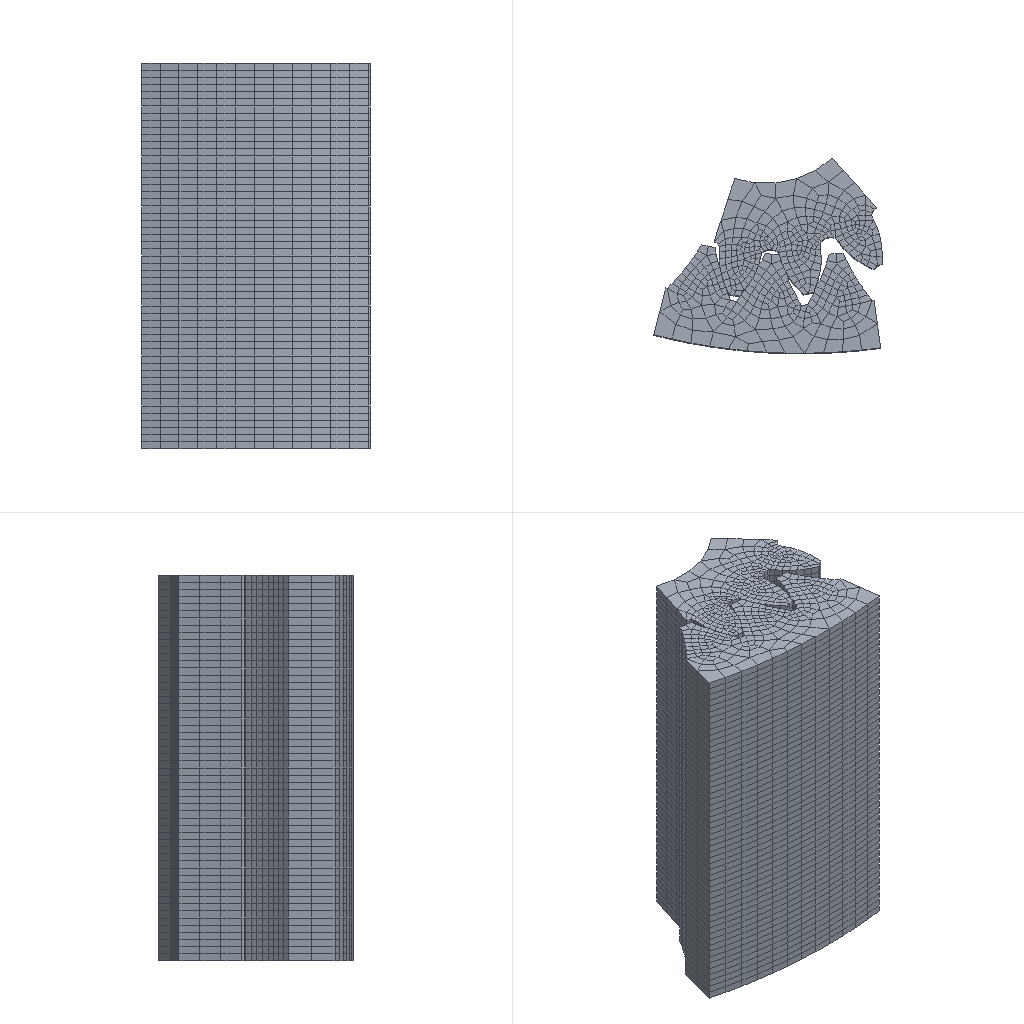Simulation study | abaqus
Set-up summary:
category,name,step,type,value,unit,region
solver,abaqus
solver,version,,,Abaqus/Standard 2020
units,not stated in the deck,,not stated
analysis,deck,,static,static
load_step,Step-1,Step-1,static
load_step,requested,,,1
mesh,nodes,,,31130
mesh,elements,,,26406
element_type,C3D8R,,solid,26406
load,load commands in deck,,count,1
bc,support commands in deck,,count,6
material,MATERIAL-1,,in results
check,setup vs results,,match,"per instance, exact: element labels, types and connectivity; labels of the nodes the elements use; coordinates of those nodes at SINGLE_PRECISION in 1 of 2 instance(s)"
Abaqus input file, long lists of numbers shortened:
*Heading
** Job name: Job-1 Model name: Model-1
** Generated by: Abaqus/CAE 2020
*Preprint, echo=NO, model=NO, history=NO, contact=NO
**
** PARTS
**
*Part, name=work-1
*Node
      1,  -37.365,   11.966,         13.5
      2,  -34.285,   8.516,         13.5
** (17378 more lines like these left out)
*Element, type=C3D8R
    1,    52,    85,    55,     2,   368,   401,   371,   318
    2,    55,    85,   265,   199,   371,   401,   581,   515
** (14956 more lines like these left out)
*Nset, nset=Set-1, generate
     1,  17380,      1
*Elset, elset=Set-1, generate
     1,  14958,      1
** Section: Section-1
*Solid Section, elset=Set-1, material=Material-1
,
*End Part
**
*Part, name=work-2
*Node
      1,  -45.957,  -1.201,        -13.5
      2,  -41.979,  -1.625,        -13.5
** (13748 more lines like these left out)
*Element, type=C3D8R
    1,   202,   195,   204,   210,   452,   445,   454,   460
    2,    76,   245,   183,   230,   326,   495,   433,   480
** (11446 more lines like these left out)
*Nset, nset=Set-1, generate
     1,  13750,      1
*Elset, elset=Set-1, generate
     1,  11448,      1
** Section: Section-1
*Solid Section, elset=Set-1, material=Material-1
,
*End Part
**
**
** ASSEMBLY
**
*Assembly, name=Assembly
**
*Instance, name=work-1-1, part=work-1
*End Instance
**
*Instance, name=work-2-1, part=work-2
*End Instance
**
*Node
      1,  -42.027,   17.188, 6.75015599e-14
*Nset, nset=Set-1, instance=work-2-1
     1,     2,     3,     4,     5,    29,    30,    31,    32,    33,    34,    35,    36,   251,   252,   253
   254,   255,   279,   280,   281,   282,   283,   284,   285,   286,   501,   502,   503,   504,   505,   529
** (43 more lines like these left out)
*Elset, elset=Set-1, instance=work-2-1
    26,   161,   167,   175,   177,   188,   191,   192,   196,   200,   205,   207,   238,   373,   379,   387
   389,   400,   403,   404,   408,   412,   417,   419,   450,   585,   591,   599,   601,   612,   615,   616
** (39 more lines like these left out)
*Nset, nset=Set-3
 1,
*Nset, nset=Set-4
 1,
*Nset, nset=Set-5, instance=work-1-1
     1,     2,     3,     4,     5,     6,     7,     8,     9,    10,    11,    12,    13,    14,    15,    16
    17,    18,    19,    20,    21,    22,    23,    24,    25,    26,    27,    28,    29,    30,    31,    32
** (38 more lines like these left out)
*Elset, elset=Set-5, instance=work-1-1
     1,     2,     3,     4,     5,     6,     7,     8,     9,    10,    11,    12,    13,    14,    15,    16
    17,    18,    19,    20,    21,    22,    23,    24,    25,    26,    27,    28,    29,    30,    31,    32
** (33 more lines like these left out)
*Nset, nset=Set-6
 1,
*Nset, nset=m_Set-2
 1,
*Elset, elset=_m_Surf-2_S6, internal, instance=work-1-1
     1,     5,     7,    11,    20,    21,    25,    39,    89,   105,   112,   161,   260,   278,   282,   284
   288,   297,   298,   302,   316,   366,   382,   389,   438,   537,   555,   559,   561,   565,   574,   575
** (42 more lines like these left out)
*Elset, elset=_m_Surf-2_S5, internal, instance=work-1-1
    11,    14,    17,    21,    26,    31,    33,    39,    56,    57,    59,    61,    62,    84,    89,    94
    95,   107,   110,   116,   120,   160,   161,   288,   291,   294,   298,   303,   308,   310,   316,   333
** (76 more lines like these left out)
*Elset, elset=_m_Surf-2_S3, internal, instance=work-1-1
    10,    16,    19,    27,    50,    58,    71,   162,   287,   293,   296,   304,   327,   335,   348,   439
   564,   570,   573,   581,   604,   612,   625,   716,   841,   847,   850,   858,   881,   889,   902,   993
** (25 more lines like these left out)
*Elset, elset=_m_Surf-2_S4, internal, instance=work-1-1
    12,    29,    34,    41,    44,    49,    51,    52,    53,    64,    65,    68,    70,    72,    80,    82
    96,    97,   108,   109,   289,   306,   311,   318,   321,   326,   328,   329,   330,   341,   342,   345
** (66 more lines like these left out)
*Surface, type=ELEMENT, name=m_Surf-2
_m_Surf-2_S6, S6
_m_Surf-2_S5, S5
_m_Surf-2_S4, S4
_m_Surf-2_S3, S3
*Elset, elset=_s_Surf-1_S6, internal, instance=work-1-1, generate
    22,  14703,    277
*Elset, elset=_s_Surf-1_S5, internal, instance=work-1-1, generate
    46,  14727,    277
*Elset, elset=_s_Surf-1_S4, internal, instance=work-1-1, generate
   249,  14930,    277
*Elset, elset=_s_Surf-1_S3, internal, instance=work-1-1
   252,   257,   529,   534,   806,   811,  1083,  1088,  1360,  1365,  1637,  1642,  1914,  1919,  2191,  2196
  2468,  2473,  2745,  2750,  3022,  3027,  3299,  3304,  3576,  3581,  3853,  3858,  4130,  4135,  4407,  4412
** (5 more lines like these left out)
*Surface, type=ELEMENT, name=s_Surf-1
_s_Surf-1_S6, S6
_s_Surf-1_S5, S5
_s_Surf-1_S4, S4
_s_Surf-1_S3, S3
*Elset, elset=_s_Surf-2_S5, internal, instance=work-2-1
    35,    45,    55,    69,    73,    80,    84,   247,   257,   267,   281,   285,   292,   296,   459,   469
   479,   493,   497,   504,   508,   671,   681,   691,   705,   709,   716,   720,   883,   893,   903,   917
** (22 more lines like these left out)
*Elset, elset=_s_Surf-2_S4, internal, instance=work-2-1
     3,     4,    11,    15,    22,    23,    25,    39,    49,    67,    68,    70,    73,   215,   216,   223
   227,   234,   235,   237,   251,   261,   279,   280,   282,   285,   427,   428,   435,   439,   446,   447
** (42 more lines like these left out)
*Elset, elset=_s_Surf-2_S3, internal, instance=work-2-1
     7,    10,    14,    20,    30,    38,    40,    41,    42,    48,    50,    51,    52,    59,    61,    62
    71,    72,    74,    75,    76,   219,   222,   226,   232,   242,   250,   252,   253,   254,   260,   262
** (69 more lines like these left out)
*Elset, elset=_s_Surf-2_S6, internal, instance=work-2-1
     5,     6,    12,    13,    19,    21,    35,    36,    45,    46,    55,    57,    71,    72,   102,   217
   218,   224,   225,   231,   233,   247,   248,   257,   258,   267,   269,   283,   284,   314,   429,   430
** (49 more lines like these left out)
*Surface, type=ELEMENT, name=s_Surf-2
_s_Surf-2_S5, S5
_s_Surf-2_S4, S4
_s_Surf-2_S6, S6
_s_Surf-2_S3, S3
** Constraint: Constraint-1
*Coupling, constraint name=Constraint-1, ref node=m_Set-2, surface=s_Surf-1
*Kinematic
*End Assembly
*Amplitude, name=Amp-1
             0.,              0.,              1.,              1.
**
** MATERIALS
**
*Material, name=Material-1
*Density
 7.8e-09,
*Elastic
206000., 0.3
*Plastic
250.,0.
**
** INTERACTION PROPERTIES
**
*Surface Interaction, name=IntProp-1
1.,
*Friction, slip tolerance=0.005
 0.15,
*Surface Behavior, pressure-overclosure=HARD
**
** INTERACTIONS
**
** Interaction: Int-1
*Contact Pair, interaction=IntProp-1, type=SURFACE TO SURFACE, adjust=0.1
s_Surf-2, m_Surf-2
** ----------------------------------------------------------------
**
** STEP: Step-1
**
*Step, name=Step-1, nlgeom=YES, inc=1000
*Static, stabilize=0.0002, allsdtol=0.05, continue=NO
0.01, 1., 1e-05, 1.
**
** BOUNDARY CONDITIONS
**
** Name: BC-1 Type: 对称/反对称/完全固定
*Boundary
Set-1, ENCASTRE
** Name: BC-2 Type: 位移/转角
*Boundary
Set-6, 1, 1
Set-6, 2, 2
Set-6, 3, 3
Set-6, 4, 4
Set-6, 5, 5
**
** LOADS
**
** Name: Load-1   Type: Moment
*Cload, amplitude=Amp-1
Set-4, 6, 5000.
**
** OUTPUT REQUESTS
**
*Restart, write, frequency=0
**
** FIELD OUTPUT: F-Output-1
**
*Output, field
*Node Output
CF, RF, RM, RT, U, V
*Element Output, directions=YES
E, LE, MISES, MISESMAX, PE, PEEQ, PEEQMAX, PEEQT, PEMAG, S, SF, YIELDPOT
*Contact Output
CDISP, CSTRESS
**
** HISTORY OUTPUT: H-Output-1
**
*Output, history, variable=PRESELECT
*End Step
Results summary:
result,step,,completed,increments=73 time=1.0/1.0
result,analysis,,,static
result,last_loadstep,,,1
result,primary field,,,U
result,reaction total,,FX,0.1517,model units
result,reaction total,,FY,0.02925,model units
result,reaction total,,FZ,1e-06,model units